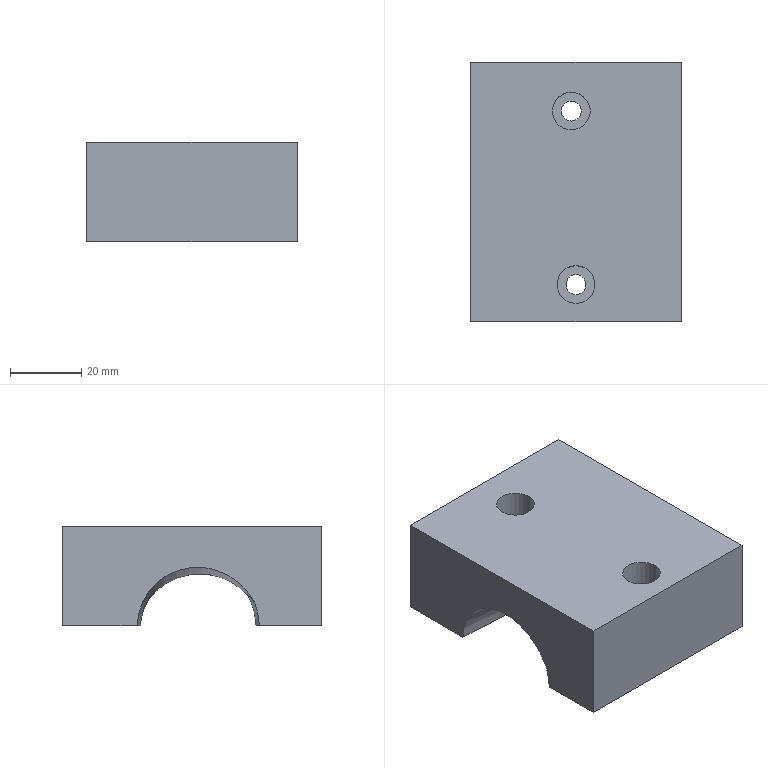Part | 1 solid | 24 faces | box 59.014 x 72.744 x 27.972 mm | volume 90143 mm3 | plane 11 | spline 7 | cylinder 6 | commonest cylinder face diameters 5.6 x2 6 x2 10.6 x2